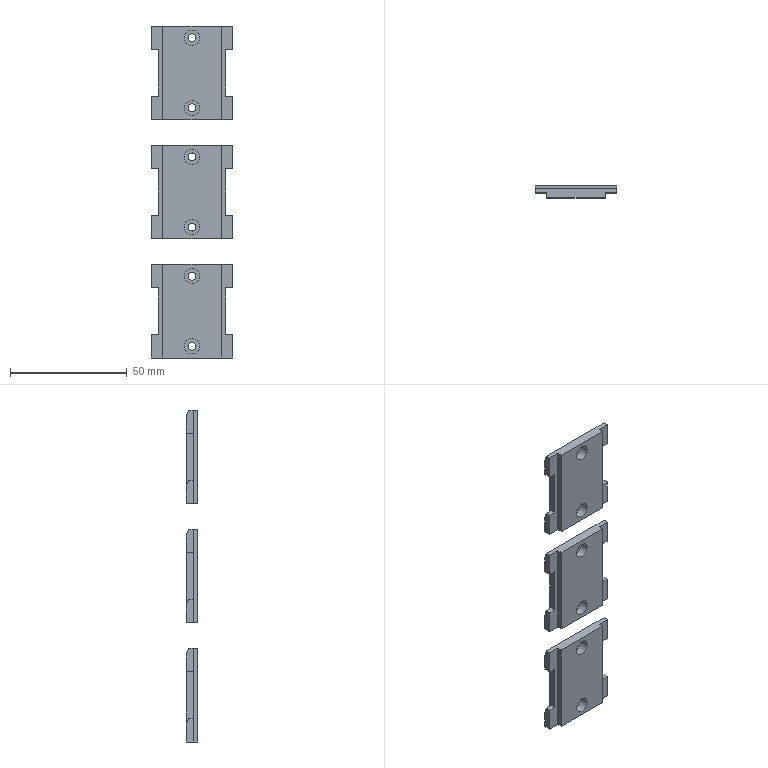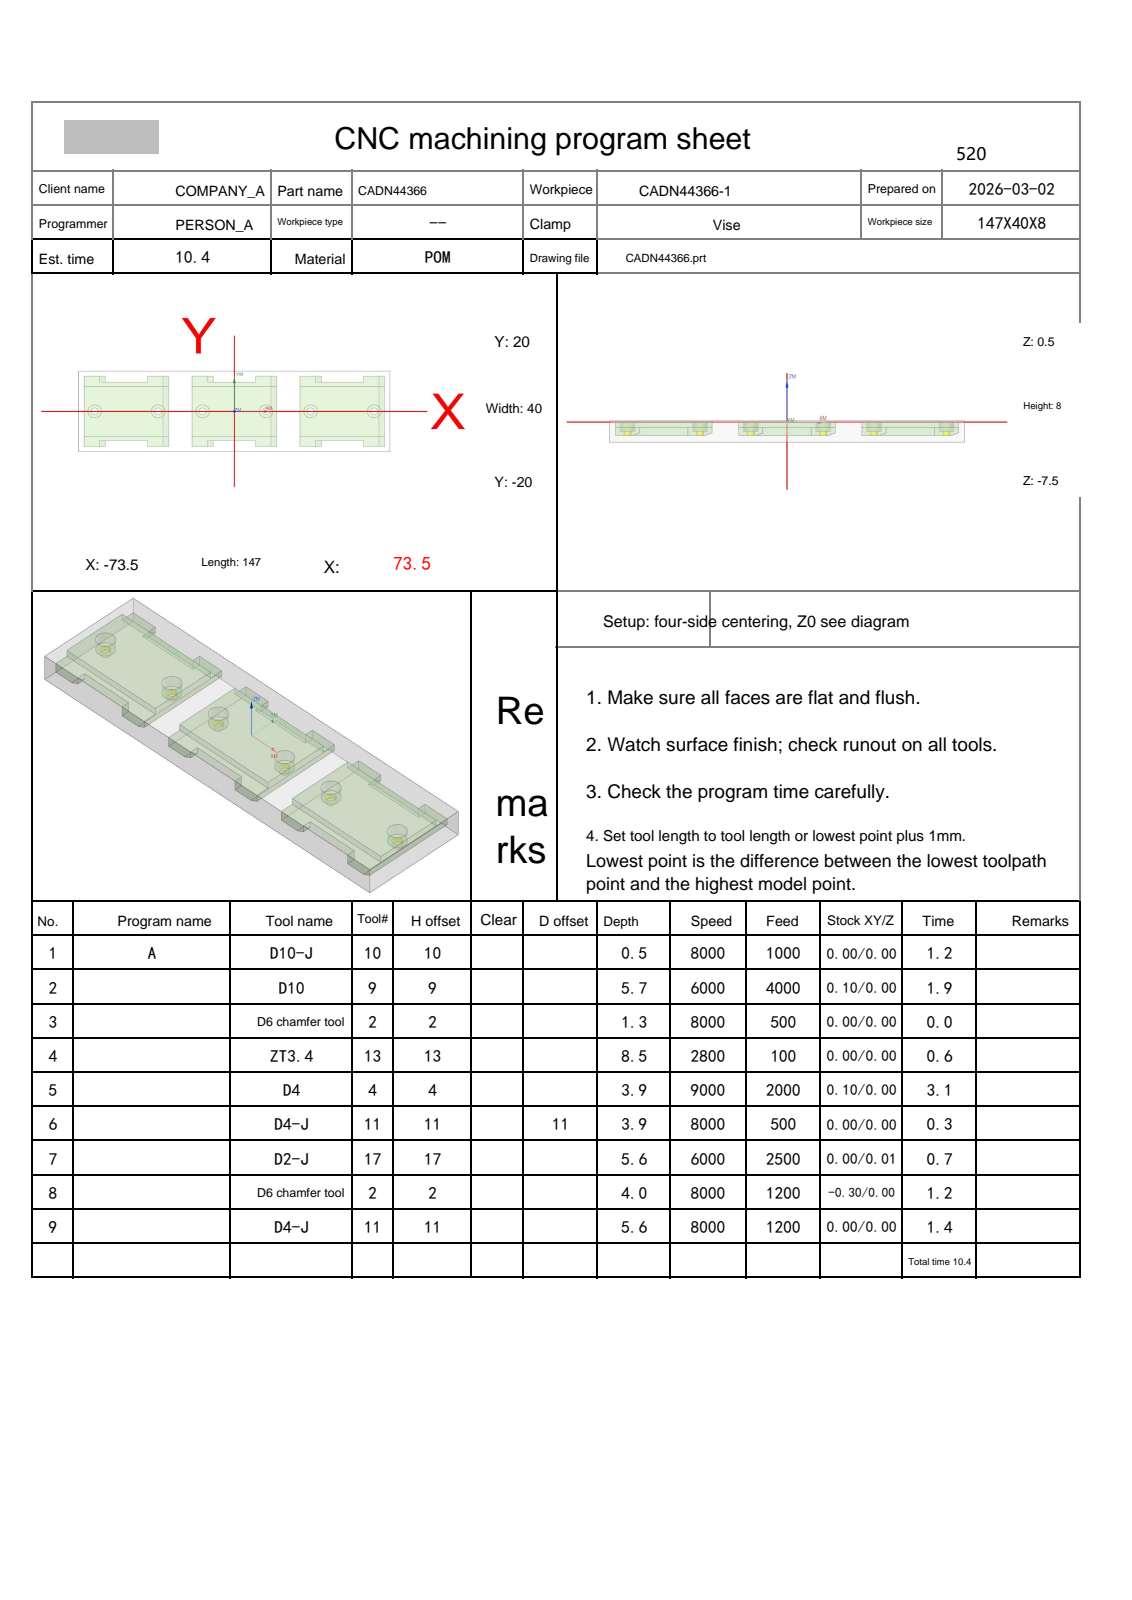NC program | NX | posted by the shop | part box 35 x 5 x 142 mm
Lines 4810 to 5584 of 5584:
N8 T02 M06
(D6 chamfer tool  D=6. R=0. H=02 ce=0.00 di=0.00)
G00 G90 G54 X-50.75 Y-14.628 M03 S6000
G43 H02 Z30.
M08
Z2.099
G01 Z-1.5 F1200.
G03 X-50.67 Y-14.328 I-.52 J.3
X-50.97 Y-13.808 I-.6 J0.0
G01 X-51. Y-13.8
X-71.
G02 X-72.3 Y-12.5 I0.0 J1.3
G01 Y12.5
G02 X-71. Y13.8 I1.3 J0.0
G01 X-31.
G02 X-29.7 Y12.5 I0.0 J-1.3
G01 Y-12.5
G02 X-31. Y-13.8 I-1.3 J0.0
G01 X-51.
X-51.03 Y-13.808
G03 X-51.33 Y-14.328 I.3 J-.52
X-51.25 Y-14.628 I.6 J0.0
G01 Z2.099
G00 Z30.
X-.25 Y14.628
Z2.099
G01 Z-1.5
G03 X-.33 Y14.328 I.52 J-.3
X-.03 Y13.808 I.6 J0.0
G01 X0.0 Y13.8
X20.
G02 X21.3 Y12.5 I0.0 J-1.3
G01 Y-12.5
G02 X20. Y-13.8 I-1.3 J0.0
G01 X-20.
G02 X-21.3 Y-12.5 I0.0 J1.3
G01 Y12.5
G02 X-20. Y13.8 I1.3 J0.0
G01 X0.0
X.03 Y13.808
G03 X.33 Y14.328 I-.3 J.52
X.25 Y14.628 I-.6 J0.0
G01 Z2.099
G00 Z30.
X50.75
Z2.099
G01 Z-1.5
G03 X50.67 Y14.328 I.52 J-.3
X50.97 Y13.808 I.6 J0.0
G01 X51. Y13.8
X71.
G02 X72.3 Y12.5 I0.0 J-1.3
G01 Y-12.5
G02 X71. Y-13.8 I-1.3 J0.0
G01 X31.
G02 X29.7 Y-12.5 I0.0 J1.3
G01 Y12.5
G02 X31. Y13.8 I1.3 J0.0
G01 X51.
X51.03 Y13.808
G03 X51.33 Y14.328 I-.3 J.52
X51.25 Y14.628 I-.6 J0.0
G01 Z2.099
G00 Z30.
X73.128 Y-15.532
Z1.755
G01 Z-3.499
G03 X72.828 Y-15.451 I-.3 J-.52
X72.308 Y-15.751 I0.0 J-.6
G01 X72.3 Y-15.781
Y-17.5
G02 X71. Y-18.8 I-1.3 J0.0
G01 X61.
G02 X59.7 Y-17.5 I0.0 J1.3
G01 Y-16.039
X59.598 Y-16.017
X59.567 Y-16.018
G03 X59.148 Y-16.59 I.181 J-.572
G01 X59.177 Y-16.771
Z.404
G00 Z30.
X42.631 Y-15.939
Z1.755
G01 Z-3.499
X42.511 Y-15.907
G03 X42.303 Y-16.027 I0.0 J-.24
G01 X42.3 Y-16.039
Y-17.5
G02 X41. Y-18.8 I-1.3 J0.0
G01 X31.
G02 X29.7 Y-17.5 I0.0 J1.3
G01 Y-15.781
X29.692 Y-15.751
G03 X29.172 Y-15.451 I-.52 J-.3
X28.872 Y-15.532 I0.0 J-.6
G01 Z1.755
G00 Z30.
Y15.532
Z1.755
G01 Z-3.499
G03 X29.172 Y15.451 I.3 J.52
X29.692 Y15.751 I0.0 J.6
G01 X29.7 Y15.781
Y17.5
G02 X31. Y18.8 I1.3 J0.0
G01 X41.
G02 X42.3 Y17.5 I0.0 J-1.3
G01 Y16.039
X42.402 Y16.017
X42.433 Y16.018
G03 X42.852 Y16.59 I-.181 J.572
G01 X42.823 Y16.771
Z.404
G00 Z30.
X59.369 Y15.939
Z1.755
G01 Z-3.499
X59.489 Y15.907
G03 X59.697 Y16.027 I0.0 J.24
G01 X59.7 Y16.039
Y17.5
G02 X61. Y18.8 I1.3 J0.0
G01 X71.
G02 X72.3 Y17.5 I0.0 J-1.3
G01 Y15.781
X72.308 Y15.751
G03 X72.828 Y15.451 I.52 J.3
X73.128 Y15.532 I0.0 J.6
G01 Z1.755
G00 Z30.
X-22.128
Z1.755
G01 Z-3.499
G03 X-21.828 Y15.451 I.3 J.52
X-21.308 Y15.751 I0.0 J.6
G01 X-21.3 Y15.781
Y17.5
G02 X-20. Y18.8 I1.3 J0.0
G01 X-10.
G02 X-8.7 Y17.5 I0.0 J-1.3
G01 Y16.039
X-8.598 Y16.017
X-8.567 Y16.018
G03 X-8.148 Y16.59 I-.181 J.572
G01 X-8.177 Y16.771
Z.404
G00 Z30.
X8.369 Y15.939
Z1.755
G01 Z-3.499
X8.489 Y15.907
G03 X8.697 Y16.027 I0.0 J.24
G01 X8.7 Y16.039
Y17.5
G02 X10. Y18.8 I1.3 J0.0
G01 X20.
G02 X21.3 Y17.5 I0.0 J-1.3
G01 Y15.781
X21.308 Y15.751
G03 X21.828 Y15.451 I.52 J.3
X22.128 Y15.532 I0.0 J.6
G01 Z1.755
G00 Z30.
Y-15.532
Z1.755
G01 Z-3.499
G03 X21.828 Y-15.451 I-.3 J-.52
X21.308 Y-15.751 I0.0 J-.6
G01 X21.3 Y-15.781
Y-17.5
G02 X20. Y-18.8 I-1.3 J0.0
G01 X10.
G02 X8.7 Y-17.5 I0.0 J1.3
G01 Y-16.039
X8.598 Y-16.017
X8.567 Y-16.018
G03 X8.148 Y-16.59 I.181 J-.572
G01 X8.177 Y-16.771
Z.404
G00 Z30.
X-8.369 Y-15.939
Z1.755
G01 Z-3.499
X-8.489 Y-15.907
G03 X-8.697 Y-16.027 I0.0 J-.24
G01 X-8.7 Y-16.039
Y-17.5
G02 X-10. Y-18.8 I-1.3 J0.0
G01 X-20.
G02 X-21.3 Y-17.5 I0.0 J1.3
G01 Y-15.781
X-21.308 Y-15.751
G03 X-21.828 Y-15.451 I-.52 J-.3
X-22.128 Y-15.532 I0.0 J-.6
G01 Z1.755
G00 Z30.
X-73.128 Y15.532
Z1.755
G01 Z-3.499
G03 X-72.828 Y15.451 I.3 J.52
X-72.308 Y15.751 I0.0 J.6
G01 X-72.3 Y15.781
Y17.5
G02 X-71. Y18.8 I1.3 J0.0
G01 X-61.
G02 X-59.7 Y17.5 I0.0 J-1.3
G01 Y16.039
X-59.598 Y16.017
X-59.567 Y16.018
G03 X-59.148 Y16.59 I-.181 J.572
G01 X-59.177 Y16.771
Z.404
G00 Z30.
X-42.631 Y15.939
Z1.755
G01 Z-3.499
X-42.511 Y15.907
G03 X-42.303 Y16.027 I0.0 J.24
G01 X-42.3 Y16.039
Y17.5
G02 X-41. Y18.8 I1.3 J0.0
G01 X-31.
G02 X-29.7 Y17.5 I0.0 J-1.3
G01 Y15.781
X-29.692 Y15.751
G03 X-29.172 Y15.451 I.52 J.3
X-28.872 Y15.532 I0.0 J.6
G01 Z1.755
G00 Z30.
Y-15.532
Z1.755
G01 Z-3.499
G03 X-29.172 Y-15.451 I-.3 J-.52
X-29.692 Y-15.751 I0.0 J-.6
G01 X-29.7 Y-15.781
Y-17.5
G02 X-31. Y-18.8 I-1.3 J0.0
G01 X-41.
G02 X-42.3 Y-17.5 I0.0 J1.3
G01 Y-16.039
X-42.402 Y-16.017
X-42.433 Y-16.018
G03 X-42.852 Y-16.59 I.181 J-.572
G01 X-42.823 Y-16.771
Z.404
G00 Z30.
X-59.369 Y-15.939
Z1.755
G01 Z-3.499
X-59.489 Y-15.907
G03 X-59.697 Y-16.027 I0.0 J-.24
G01 X-59.7 Y-16.039
Y-17.5
G02 X-61. Y-18.8 I-1.3 J0.0
G01 X-71.
G02 X-72.3 Y-17.5 I0.0 J1.3
G01 Y-15.781
X-72.308 Y-15.751
G03 X-72.828 Y-15.451 I-.52 J-.3
X-73.128 Y-15.532 I0.0 J-.6
G01 Z1.755
G00 Z30.
G00 G90 X63.937 Y1.497 M03 S8000
Z30.
Z2.5
G01 X63.892 Y1.44 Z2.474 F500.
X63.719 Y1.147 Z2.35
X63.587 Y.834 Z2.226
X63.498 Y.507 Z2.103
X63.453 Y.17 Z1.979
Y-.17 Z1.855
X63.498 Y-.507 Z1.732
X63.587 Y-.834 Z1.608
X63.719 Y-1.147 Z1.484
X63.892 Y-1.44 Z1.361
X64.102 Y-1.707 Z1.237
X64.345 Y-1.944 Z1.113
X64.618 Y-2.147 Z.99
X64.832 Y-2.27 Z.9
X65.144 Y-2.405 Z.776
X65.471 Y-2.498 Z.652
X65.807 Y-2.546 Z.529
X66.147 Y-2.549 Z.405
X66.484 Y-2.507 Z.281
X66.812 Y-2.42 Z.158
X67.127 Y-2.291 Z.034
X67.421 Y-2.121 Z-.089
X67.69 Y-1.914 Z-.213
X67.929 Y-1.672 Z-.337
X68.134 Y-1.402 Z-.46
X68.301 Y-1.106 Z-.584
X68.428 Y-.79 Z-.708
X68.511 Y-.461 Z-.831
X68.55 Y-.124 Z-.955
Y0.0 Z-1.
G03 X66. Y2.55 I-2.55 J0.0
X63.45 Y0.0 I0.0 J-2.55
X66. Y-2.55 I2.55 J0.0
X68.55 Y0.0 I0.0 J2.55
X68.501 Y.497 I-2.55 J0.0
G01 Z1.5
G00 Z30.
X33.937 Y1.497
Z2.5
G01 X33.892 Y1.44 Z2.474
X33.719 Y1.147 Z2.35
X33.587 Y.834 Z2.226
X33.498 Y.507 Z2.103
X33.453 Y.17 Z1.979
Y-.17 Z1.855
X33.498 Y-.507 Z1.732
X33.587 Y-.834 Z1.608
X33.719 Y-1.147 Z1.484
X33.892 Y-1.44 Z1.361
X34.102 Y-1.707 Z1.237
X34.345 Y-1.944 Z1.113
X34.618 Y-2.147 Z.99
X34.832 Y-2.27 Z.9
X35.144 Y-2.405 Z.776
X35.471 Y-2.498 Z.652
X35.807 Y-2.546 Z.529
X36.147 Y-2.549 Z.405
X36.484 Y-2.507 Z.281
X36.812 Y-2.42 Z.158
X37.127 Y-2.291 Z.034
X37.421 Y-2.121 Z-.089
X37.69 Y-1.914 Z-.213
X37.929 Y-1.672 Z-.337
X38.134 Y-1.402 Z-.46
X38.301 Y-1.106 Z-.584
X38.428 Y-.79 Z-.708
X38.511 Y-.461 Z-.831
X38.55 Y-.124 Z-.955
Y0.0 Z-1.
G03 X36. Y2.55 I-2.55 J0.0
X33.45 Y0.0 I0.0 J-2.55
X36. Y-2.55 I2.55 J0.0
X38.55 Y0.0 I0.0 J2.55
X38.501 Y.497 I-2.55 J0.0
G01 Z1.5
G00 Z30.
X12.937 Y1.497
Z2.5
G01 X12.892 Y1.44 Z2.474
X12.719 Y1.147 Z2.35
X12.587 Y.834 Z2.226
X12.498 Y.507 Z2.103
X12.453 Y.17 Z1.979
Y-.17 Z1.855
X12.498 Y-.507 Z1.732
X12.587 Y-.834 Z1.608
X12.719 Y-1.147 Z1.484
X12.892 Y-1.44 Z1.361
X13.102 Y-1.707 Z1.237
X13.345 Y-1.944 Z1.113
X13.618 Y-2.147 Z.99
X13.832 Y-2.27 Z.9
X14.144 Y-2.405 Z.776
X14.471 Y-2.498 Z.652
X14.807 Y-2.546 Z.529
X15.147 Y-2.549 Z.405
X15.484 Y-2.507 Z.281
X15.812 Y-2.42 Z.158
X16.127 Y-2.291 Z.034
X16.421 Y-2.121 Z-.089
X16.69 Y-1.914 Z-.213
X16.929 Y-1.672 Z-.337
X17.134 Y-1.402 Z-.46
X17.301 Y-1.106 Z-.584
X17.428 Y-.79 Z-.708
X17.511 Y-.461 Z-.831
X17.55 Y-.124 Z-.955
Y0.0 Z-1.
G03 X15. Y2.55 I-2.55 J0.0
X12.45 Y0.0 I0.0 J-2.55
X15. Y-2.55 I2.55 J0.0
X17.55 Y0.0 I0.0 J2.55
X17.501 Y.497 I-2.55 J0.0
G01 Z1.5
G00 Z30.
X-17.063 Y1.497
Z2.5
G01 X-17.108 Y1.44 Z2.474
X-17.281 Y1.147 Z2.35
X-17.413 Y.834 Z2.226
X-17.502 Y.507 Z2.103
X-17.547 Y.17 Z1.979
Y-.17 Z1.855
X-17.502 Y-.507 Z1.732
X-17.413 Y-.834 Z1.608
X-17.281 Y-1.147 Z1.484
X-17.108 Y-1.44 Z1.361
X-16.898 Y-1.707 Z1.237
X-16.655 Y-1.944 Z1.113
X-16.382 Y-2.147 Z.99
X-16.168 Y-2.27 Z.9
X-15.856 Y-2.405 Z.776
X-15.529 Y-2.498 Z.652
X-15.193 Y-2.546 Z.529
X-14.853 Y-2.549 Z.405
X-14.516 Y-2.507 Z.281
X-14.188 Y-2.42 Z.158
X-13.873 Y-2.291 Z.034
X-13.579 Y-2.121 Z-.089
X-13.31 Y-1.914 Z-.213
X-13.071 Y-1.672 Z-.337
X-12.866 Y-1.402 Z-.46
X-12.699 Y-1.106 Z-.584
X-12.572 Y-.79 Z-.708
X-12.489 Y-.461 Z-.831
X-12.45 Y-.124 Z-.955
Y0.0 Z-1.
G03 X-15. Y2.55 I-2.55 J0.0
X-17.55 Y0.0 I0.0 J-2.55
X-15. Y-2.55 I2.55 J0.0
X-12.45 Y0.0 I0.0 J2.55
X-12.499 Y.497 I-2.55 J0.0
G01 Z1.5
G00 Z30.
X-38.063 Y1.497
Z2.5
G01 X-38.108 Y1.44 Z2.474
X-38.281 Y1.147 Z2.35
X-38.413 Y.834 Z2.226
X-38.502 Y.507 Z2.103
X-38.547 Y.17 Z1.979
Y-.17 Z1.855
X-38.502 Y-.507 Z1.732
X-38.413 Y-.834 Z1.608
X-38.281 Y-1.147 Z1.484
X-38.108 Y-1.44 Z1.361
X-37.898 Y-1.707 Z1.237
X-37.655 Y-1.944 Z1.113
X-37.382 Y-2.147 Z.99
X-37.168 Y-2.27 Z.9
X-36.856 Y-2.405 Z.776
X-36.529 Y-2.498 Z.652
X-36.193 Y-2.546 Z.529
X-35.853 Y-2.549 Z.405
X-35.516 Y-2.507 Z.281
X-35.188 Y-2.42 Z.158
X-34.873 Y-2.291 Z.034
X-34.579 Y-2.121 Z-.089
X-34.31 Y-1.914 Z-.213
X-34.071 Y-1.672 Z-.337
X-33.866 Y-1.402 Z-.46
X-33.699 Y-1.106 Z-.584
X-33.572 Y-.79 Z-.708
X-33.489 Y-.461 Z-.831
X-33.45 Y-.124 Z-.955
Y0.0 Z-1.
G03 X-36. Y2.55 I-2.55 J0.0
X-38.55 Y0.0 I0.0 J-2.55
X-36. Y-2.55 I2.55 J0.0
X-33.45 Y0.0 I0.0 J2.55
X-33.499 Y.497 I-2.55 J0.0
G01 Z1.5
G00 Z30.
X-68.063 Y1.497
Z2.5
G01 X-68.108 Y1.44 Z2.474
X-68.281 Y1.147 Z2.35
X-68.413 Y.834 Z2.226
X-68.502 Y.507 Z2.103
X-68.547 Y.17 Z1.979
Y-.17 Z1.855
X-68.502 Y-.507 Z1.732
X-68.413 Y-.834 Z1.608
X-68.281 Y-1.147 Z1.484
X-68.108 Y-1.44 Z1.361
X-67.898 Y-1.707 Z1.237
X-67.655 Y-1.944 Z1.113
X-67.382 Y-2.147 Z.99
X-67.168 Y-2.27 Z.9
X-66.856 Y-2.405 Z.776
X-66.529 Y-2.498 Z.652
X-66.193 Y-2.546 Z.529
X-65.853 Y-2.549 Z.405
X-65.516 Y-2.507 Z.281
X-65.188 Y-2.42 Z.158
X-64.873 Y-2.291 Z.034
X-64.579 Y-2.121 Z-.089
X-64.31 Y-1.914 Z-.213
X-64.071 Y-1.672 Z-.337
X-63.866 Y-1.402 Z-.46
X-63.699 Y-1.106 Z-.584
X-63.572 Y-.79 Z-.708
X-63.489 Y-.461 Z-.831
X-63.45 Y-.124 Z-.955
Y0.0 Z-1.
G03 X-66. Y2.55 I-2.55 J0.0
X-68.55 Y0.0 I0.0 J-2.55
X-66. Y-2.55 I2.55 J0.0
X-63.45 Y0.0 I0.0 J2.55
X-63.499 Y.497 I-2.55 J0.0
G01 Z1.5
G00 Z30.
G91 G28 Z0.0
M05
M09
G91 G28 Z0.0
M01
N9 T11 M06
(D4-J  D=4. R=0. H=11 ce=0.30 di=0.00)
G00 G90 G54 X-51. Y19.5 M03 S8000
G43 H11 Z30.
M08
Z-1.5
G01 Z-2. F1200.
Y14.9
X-41.4
Y17.9
X-30.6
Y14.8
X-71.4
Y17.9
X-60.6
Y14.9
X-51.
X-50.5
Y19.5
Z-1.5
G00 Z30.
X-51. Y-19.5
Z-1.5
G01 Z-2.
Y-14.9
X-60.6
Y-17.9
X-71.4
Y-14.8
X-30.6
Y-17.9
X-41.4
Y-14.9
X-51.
X-51.5
Y-19.5
Z-1.5
G00 Z30.
X0.0
Z-1.5
G01 Z-2.
Y-14.9
X-9.6
Y-17.9
X-20.4
Y-14.8
X20.4
Y-17.9
X9.6
Y-14.9
X0.0
X-.5
Y-19.5
Z-1.5
G00 Z30.
X0.0 Y19.5
Z-1.5
G01 Z-2.
Y14.9
X9.6
Y17.9
X20.4
Y14.8
X-20.4
Y17.9
X-9.6
Y14.9
X0.0
X.5
Y19.5
Z-1.5
G00 Z30.
X51.
Z-1.5
G01 Z-2.
Y14.9
X60.6
Y17.9
X71.4
Y14.8
X30.6
Y17.9
X41.4
Y14.9
X51.
X51.5
Y19.5
Z-1.5
G00 Z30.
X51. Y-19.5
Z-1.5
G01 Z-2.
Y-14.9
X41.4
Y-17.9
X30.6
Y-14.8
X71.4
Y-17.9
X60.6
Y-14.9
X51.
X50.5
Y-19.5
Z-1.5
G00 Z30.
G00 G90 X-28.2 Y-15.6 M03 S8000
Z30.
Z-1.495
G01 Z-1.995 F1200.
G41 D11
Y-15.5
G03 X-29.2 Y-14.5 I-1. J0.0
G01 X-72.8
G03 X-73.8 Y-15.5 I0.0 J-1.
G01 G40 Y-15.6
Z-1.495
G00 Z30.
Y15.6
Z-1.495
G01 Z-1.995
G41 D11
Y15.5
G03 X-72.8 Y14.5 I1. J0.0
G01 X-29.2
G03 X-28.2 Y15.5 I0.0 J1.
G01 G40 Y15.6
Z-1.495
G00 Z30.
X-22.8
Z-1.495
G01 Z-1.995
G41 D11
Y15.5
G03 X-21.8 Y14.5 I1. J0.0
G01 X21.8
G03 X22.8 Y15.5 I0.0 J1.
G01 G40 Y15.6
Z-1.495
G00 Z30.
Y-15.6
Z-1.495
G01 Z-1.995
G41 D11
Y-15.5
G03 X21.8 Y-14.5 I-1. J0.0
G01 X-21.8
G03 X-22.8 Y-15.5 I0.0 J-1.
G01 G40 Y-15.6
Z-1.495
G00 Z30.
X73.8
Z-1.495
G01 Z-1.995
G41 D11
Y-15.5
G03 X72.8 Y-14.5 I-1. J0.0
G01 X29.2
G03 X28.2 Y-15.5 I0.0 J-1.
G01 G40 Y-15.6
Z-1.495
G00 Z30.
Y15.6
Z-1.495
G01 Z-1.995
G41 D11
Y15.5
G03 X29.2 Y14.5 I1. J0.0
G01 X72.8
G03 X73.8 Y15.5 I0.0 J1.
G01 G40 Y15.6
Z-1.495
G00 Z30.
G00 G90 X-73.932 Y-18.503 M03 S6000
Z30.
Z-4.6
G01 Z-5.1 F1000.
G41 D11
X-73.833 Y-18.486
G03 X-73. Y-17.5 I-.167 J.986
G01 Y17.5
G02 X-71. Y19.5 I2. J0.0
G01 X-61.
G02 X-59. Y17.5 I0.0 J-2.
G01 Y16.5
X-43.
Y17.5
G02 X-41. Y19.5 I2. J0.0
G01 X-31.
G02 X-29. Y17.5 I0.0 J-2.
G01 Y-17.5
G02 X-31. Y-19.5 I-2. J0.0
G01 X-41.
G02 X-43. Y-17.5 I0.0 J2.
G01 Y-16.5
X-59.
Y-17.5
G02 X-61. Y-19.5 I-2. J0.0
G01 X-71.
G02 X-73. Y-17.5 I0.0 J2.
G01 Y-17.
G03 X-74. Y-16. I-1. J0.0
G01 G40 X-74.1
Z-4.6
G00 Z30.
X-22.932 Y-18.503
Z-4.6
G01 Z-5.1
G41 D11
X-22.833 Y-18.486
G03 X-22. Y-17.5 I-.167 J.986
G01 Y17.5
G02 X-20. Y19.5 I2. J0.0
G01 X-10.
G02 X-8. Y17.5 I0.0 J-2.
G01 Y16.5
X8.
Y17.5
G02 X10. Y19.5 I2. J0.0
G01 X20.
G02 X22. Y17.5 I0.0 J-2.
G01 Y-17.5
G02 X20. Y-19.5 I-2. J0.0
G01 X10.
G02 X8. Y-17.5 I0.0 J2.
G01 Y-16.5
X-8.
Y-17.5
G02 X-10. Y-19.5 I-2. J0.0
G01 X-20.
G02 X-22. Y-17.5 I0.0 J2.
G01 Y-17.
G03 X-23. Y-16. I-1. J0.0
G01 G40 X-23.1
Z-4.6
G00 Z30.
X73.932 Y18.503
Z-4.6
G01 Z-5.1
G41 D11
X73.833 Y18.486
G03 X73. Y17.5 I.167 J-.986
G01 Y-17.5
G02 X71. Y-19.5 I-2. J0.0
G01 X61.
G02 X59. Y-17.5 I0.0 J2.
G01 Y-16.5
X43.
Y-17.5
G02 X41. Y-19.5 I-2. J0.0
G01 X31.
G02 X29. Y-17.5 I0.0 J2.
G01 Y17.5
G02 X31. Y19.5 I2. J0.0
G01 X41.
G02 X43. Y17.5 I0.0 J-2.
G01 Y16.5
X59.
Y17.5
G02 X61. Y19.5 I2. J0.0
G01 X71.
G02 X73. Y17.5 I0.0 J-2.
G01 Y17.
G03 X74. Y16. I1. J0.0
G01 G40 X74.1
Z-4.6
G00 Z30.
M05
M09
G91 G28 Z0.0
G91 G28 Y0.0
M30
%